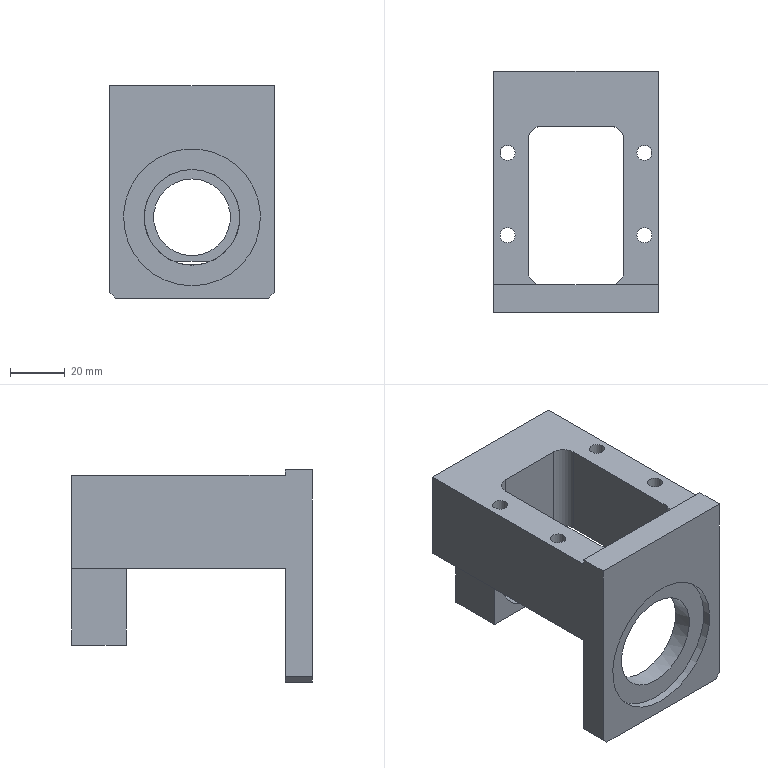Part | NX | 1 solid | 41 faces | box 60 x 88 x 77.5 mm | volume 126887 mm3 | plane 26 | cylinder 15 | commonest cylinder face diameters 5.5 x4 9 x4 10 x4 28 x1 35 x1 50 x1
STEP:
#1=CARTESIAN_POINT('',(-12.738,10.,12.));
#2=VERTEX_POINT('',#1);
#3=CARTESIAN_POINT('',(-12.5,10.,12.));
#4=VERTEX_POINT('',#3);
#5=CARTESIAN_POINT('',(30.,10.,12.));
#6=DIRECTION('',(1.,0.,0.));
#7=VECTOR('',#6,1.);
#8=LINE('',#5,#7);
#9=EDGE_CURVE('',#2,#4,#8,.T.);
#10=ORIENTED_EDGE('',*,*,#9,.T.);
#11=CARTESIAN_POINT('',(-12.5,10.,12.247));
#12=VERTEX_POINT('',#11);
#13=CARTESIAN_POINT('',(-12.5,10.,52.8));
#14=DIRECTION('',(0.,0.,-1.));
#15=VECTOR('',#14,1.);
#16=LINE('',#13,#15);
#17=EDGE_CURVE('',#12,#4,#16,.T.);
#18=ORIENTED_EDGE('',*,*,#17,.F.);
#19=CARTESIAN_POINT('',(0.,10.,0.));
#20=DIRECTION('',(0.,-1.,0.));
#21=DIRECTION('',(0.,0.,-1.));
#22=AXIS2_PLACEMENT_3D('',#19,#20,#21);
#23=CIRCLE('',#22,17.5);
#24=EDGE_CURVE('',#12,#2,#23,.T.);
#25=ORIENTED_EDGE('',*,*,#24,.T.);
#26=EDGE_LOOP('',(#10,#18,#25));
#27=FACE_OUTER_BOUND('',#26,.T.);
#28=CARTESIAN_POINT('',(0.,10.,0.));
#29=DIRECTION('',(0.,1.,0.));
#30=DIRECTION('',(0.,0.,-1.));
#31=AXIS2_PLACEMENT_3D('',#28,#29,#30);
#32=PLANE('',#31);
#33=ADVANCED_FACE('',(#27),#32,.F.);
#34=CARTESIAN_POINT('',(0.,88.,14.));
#35=VERTEX_POINT('',#34);
#36=CARTESIAN_POINT('',(0.,88.,0.));
#37=DIRECTION('',(0.,1.,0.));
#38=DIRECTION('',(0.,0.,1.));
#39=AXIS2_PLACEMENT_3D('',#36,#37,#38);
#40=CIRCLE('',#39,14.);
#41=EDGE_CURVE('',#35,#35,#40,.T.);
#42=ORIENTED_EDGE('',*,*,#41,.T.);
#43=EDGE_LOOP('',(#42));
#44=FACE_BOUND('',#43,.T.);
#45=CARTESIAN_POINT('',(0.,68.,14.));
#46=VERTEX_POINT('',#45);
#47=CARTESIAN_POINT('',(0.,68.,0.));
#48=DIRECTION('',(0.,-1.,0.));
#49=DIRECTION('',(0.,0.,1.));
#50=AXIS2_PLACEMENT_3D('',#47,#48,#49);
#51=CIRCLE('',#50,14.);
#52=EDGE_CURVE('',#46,#46,#51,.T.);
#53=ORIENTED_EDGE('',*,*,#52,.T.);
#54=EDGE_LOOP('',(#53));
#55=FACE_BOUND('',#54,.T.);
#56=CARTESIAN_POINT('',(0.,10.,0.));
#57=DIRECTION('',(0.,1.,0.));
#58=DIRECTION('',(0.,0.,-1.));
#59=AXIS2_PLACEMENT_3D('',#56,#57,#58);
#60=CYLINDRICAL_SURFACE('',#59,14.);
#61=ADVANCED_FACE('',(#44,#55),#60,.F.);
#62=CARTESIAN_POINT('',(12.5,10.,12.));
#63=VERTEX_POINT('',#62);
#64=CARTESIAN_POINT('',(12.738,10.,12.));
#65=VERTEX_POINT('',#64);
#66=CARTESIAN_POINT('',(30.,10.,12.));
#67=DIRECTION('',(1.,0.,0.));
#68=VECTOR('',#67,1.);
#69=LINE('',#66,#68);
#70=EDGE_CURVE('',#63,#65,#69,.T.);
#71=ORIENTED_EDGE('',*,*,#70,.T.);
#72=CARTESIAN_POINT('',(12.5,10.,12.247));
#73=VERTEX_POINT('',#72);
#74=CARTESIAN_POINT('',(0.,10.,0.));
#75=DIRECTION('',(0.,-1.,0.));
#76=DIRECTION('',(0.,0.,-1.));
#77=AXIS2_PLACEMENT_3D('',#74,#75,#76);
#78=CIRCLE('',#77,17.5);
#79=EDGE_CURVE('',#65,#73,#78,.T.);
#80=ORIENTED_EDGE('',*,*,#79,.T.);
#81=CARTESIAN_POINT('',(12.5,10.,52.8));
#82=DIRECTION('',(0.,0.,-1.));
#83=VECTOR('',#82,1.);
#84=LINE('',#81,#83);
#85=EDGE_CURVE('',#73,#63,#84,.T.);
#86=ORIENTED_EDGE('',*,*,#85,.T.);
#87=EDGE_LOOP('',(#71,#80,#86));
#88=FACE_OUTER_BOUND('',#87,.T.);
#89=CARTESIAN_POINT('',(0.,10.,0.));
#90=DIRECTION('',(0.,1.,0.));
#91=DIRECTION('',(0.,0.,-1.));
#92=AXIS2_PLACEMENT_3D('',#89,#90,#91);
#93=PLANE('',#92);
#94=ADVANCED_FACE('',(#88),#93,.F.);
#95=CARTESIAN_POINT('',(-18.,68.,12.));
#96=VERTEX_POINT('',#95);
#97=CARTESIAN_POINT('',(-18.,68.,-16.));
#98=VERTEX_POINT('',#97);
#99=CARTESIAN_POINT('',(-18.,68.,12.));
#100=DIRECTION('',(0.,0.,-1.));
#101=VECTOR('',#100,1.);
#102=LINE('',#99,#101);
#103=EDGE_CURVE('',#96,#98,#102,.T.);
#104=ORIENTED_EDGE('',*,*,#103,.F.);
#105=CARTESIAN_POINT('',(-18.,88.,12.));
#106=VERTEX_POINT('',#105);
#107=CARTESIAN_POINT('',(-18.,10.,12.));
#108=DIRECTION('',(0.,1.,0.));
#109=VECTOR('',#108,1.);
#110=LINE('',#107,#109);
#111=EDGE_CURVE('',#96,#106,#110,.T.);
#112=ORIENTED_EDGE('',*,*,#111,.T.);
#113=CARTESIAN_POINT('',(-18.,88.,-16.));
#114=VERTEX_POINT('',#113);
#115=CARTESIAN_POINT('',(-18.,88.,12.));
#116=DIRECTION('',(0.,0.,-1.));
#117=VECTOR('',#116,1.);
#118=LINE('',#115,#117);
#119=EDGE_CURVE('',#106,#114,#118,.T.);
#120=ORIENTED_EDGE('',*,*,#119,.T.);
#121=CARTESIAN_POINT('',(-18.,10.,-16.));
#122=DIRECTION('',(0.,1.,0.));
#123=VECTOR('',#122,1.);
#124=LINE('',#121,#123);
#125=EDGE_CURVE('',#98,#114,#124,.T.);
#126=ORIENTED_EDGE('',*,*,#125,.F.);
#127=EDGE_LOOP('',(#104,#112,#120,#126));
#128=FACE_OUTER_BOUND('',#127,.T.);
#129=CARTESIAN_POINT('',(-18.,10.,12.));
#130=DIRECTION('',(1.,0.,0.));
#131=DIRECTION('',(0.,0.,1.));
#132=AXIS2_PLACEMENT_3D('',#129,#130,#131);
#133=PLANE('',#132);
#134=ADVANCED_FACE('',(#128),#133,.F.);
#135=CARTESIAN_POINT('',(18.,68.,-16.));
#136=VERTEX_POINT('',#135);
#137=CARTESIAN_POINT('',(18.,68.,12.));
#138=VERTEX_POINT('',#137);
#139=CARTESIAN_POINT('',(18.,68.,-16.));
#140=DIRECTION('',(0.,0.,1.));
#141=VECTOR('',#140,1.);
#142=LINE('',#139,#141);
#143=EDGE_CURVE('',#136,#138,#142,.T.);
#144=ORIENTED_EDGE('',*,*,#143,.F.);
#145=CARTESIAN_POINT('',(18.,88.,-16.));
#146=VERTEX_POINT('',#145);
#147=CARTESIAN_POINT('',(18.,10.,-16.));
#148=DIRECTION('',(0.,1.,0.));
#149=VECTOR('',#148,1.);
#150=LINE('',#147,#149);
#151=EDGE_CURVE('',#136,#146,#150,.T.);
#152=ORIENTED_EDGE('',*,*,#151,.T.);
#153=CARTESIAN_POINT('',(18.,88.,12.));
#154=VERTEX_POINT('',#153);
#155=CARTESIAN_POINT('',(18.,88.,-16.));
#156=DIRECTION('',(0.,0.,1.));
#157=VECTOR('',#156,1.);
#158=LINE('',#155,#157);
#159=EDGE_CURVE('',#146,#154,#158,.T.);
#160=ORIENTED_EDGE('',*,*,#159,.T.);
#161=CARTESIAN_POINT('',(18.,10.,12.));
#162=DIRECTION('',(0.,1.,0.));
#163=VECTOR('',#162,1.);
#164=LINE('',#161,#163);
#165=EDGE_CURVE('',#138,#154,#164,.T.);
#166=ORIENTED_EDGE('',*,*,#165,.F.);
#167=EDGE_LOOP('',(#144,#152,#160,#166));
#168=FACE_OUTER_BOUND('',#167,.T.);
#169=CARTESIAN_POINT('',(18.,10.,-16.));
#170=DIRECTION('',(-1.,0.,0.));
#171=DIRECTION('',(0.,0.,-1.));
#172=AXIS2_PLACEMENT_3D('',#169,#170,#171);
#173=PLANE('',#172);
#174=ADVANCED_FACE('',(#168),#173,.F.);
#175=CARTESIAN_POINT('',(-17.5,63.,12.));
#176=VERTEX_POINT('',#175);
#177=CARTESIAN_POINT('',(-17.5,15.,12.));
#178=VERTEX_POINT('',#177);
#179=CARTESIAN_POINT('',(-17.5,15.,12.));
#180=DIRECTION('',(0.,-1.,0.));
#181=VECTOR('',#180,1.);
#182=LINE('',#179,#181);
#183=EDGE_CURVE('',#176,#178,#182,.T.);
#184=ORIENTED_EDGE('',*,*,#183,.F.);
#185=CARTESIAN_POINT('',(-17.5,63.,46.));
#186=VERTEX_POINT('',#185);
#187=CARTESIAN_POINT('',(-17.5,63.,52.8));
#188=DIRECTION('',(0.,0.,1.));
#189=VECTOR('',#188,1.);
#190=LINE('',#187,#189);
#191=EDGE_CURVE('',#176,#186,#190,.T.);
#192=ORIENTED_EDGE('',*,*,#191,.T.);
#193=CARTESIAN_POINT('',(-17.5,15.,46.));
#194=VERTEX_POINT('',#193);
#195=CARTESIAN_POINT('',(-17.5,10.,46.));
#196=DIRECTION('',(0.,1.,0.));
#197=VECTOR('',#196,1.);
#198=LINE('',#195,#197);
#199=EDGE_CURVE('',#194,#186,#198,.T.);
#200=ORIENTED_EDGE('',*,*,#199,.F.);
#201=CARTESIAN_POINT('',(-17.5,15.,52.8));
#202=DIRECTION('',(0.,0.,1.));
#203=VECTOR('',#202,1.);
#204=LINE('',#201,#203);
#205=EDGE_CURVE('',#178,#194,#204,.T.);
#206=ORIENTED_EDGE('',*,*,#205,.F.);
#207=EDGE_LOOP('',(#184,#192,#200,#206));
#208=FACE_OUTER_BOUND('',#207,.T.);
#209=CARTESIAN_POINT('',(-17.5,15.,52.8));
#210=DIRECTION('',(-1.,0.,0.));
#211=DIRECTION('',(0.,1.,0.));
#212=AXIS2_PLACEMENT_3D('',#209,#210,#211);
#213=PLANE('',#212);
#214=ADVANCED_FACE('',(#208),#213,.F.);
#215=CARTESIAN_POINT('',(17.5,15.,12.));
#216=VERTEX_POINT('',#215);
#217=CARTESIAN_POINT('',(17.5,63.,12.));
#218=VERTEX_POINT('',#217);
#219=CARTESIAN_POINT('',(17.5,63.,12.));
#220=DIRECTION('',(0.,1.,0.));
#221=VECTOR('',#220,1.);
#222=LINE('',#219,#221);
#223=EDGE_CURVE('',#216,#218,#222,.T.);
#224=ORIENTED_EDGE('',*,*,#223,.F.);
#225=CARTESIAN_POINT('',(17.5,15.,46.));
#226=VERTEX_POINT('',#225);
#227=CARTESIAN_POINT('',(17.5,15.,52.8));
#228=DIRECTION('',(0.,0.,1.));
#229=VECTOR('',#228,1.);
#230=LINE('',#227,#229);
#231=EDGE_CURVE('',#216,#226,#230,.T.);
#232=ORIENTED_EDGE('',*,*,#231,.T.);
#233=CARTESIAN_POINT('',(17.5,63.,46.));
#234=VERTEX_POINT('',#233);
#235=CARTESIAN_POINT('',(17.5,10.,46.));
#236=DIRECTION('',(0.,-1.,0.));
#237=VECTOR('',#236,1.);
#238=LINE('',#235,#237);
#239=EDGE_CURVE('',#234,#226,#238,.T.);
#240=ORIENTED_EDGE('',*,*,#239,.F.);
#241=CARTESIAN_POINT('',(17.5,63.,52.8));
#242=DIRECTION('',(0.,0.,1.));
#243=VECTOR('',#242,1.);
#244=LINE('',#241,#243);
#245=EDGE_CURVE('',#218,#234,#244,.T.);
#246=ORIENTED_EDGE('',*,*,#245,.F.);
#247=EDGE_LOOP('',(#224,#232,#240,#246));
#248=FACE_OUTER_BOUND('',#247,.T.);
#249=CARTESIAN_POINT('',(17.5,63.,52.8));
#250=DIRECTION('',(1.,0.,0.));
#251=DIRECTION('',(0.,-1.,0.));
#252=AXIS2_PLACEMENT_3D('',#249,#250,#251);
#253=PLANE('',#252);
#254=ADVANCED_FACE('',(#248),#253,.F.);
#255=CARTESIAN_POINT('',(-12.5,68.,12.));
#256=VERTEX_POINT('',#255);
#257=CARTESIAN_POINT('',(-12.5,63.,12.));
#258=DIRECTION('',(0.,0.,1.));
#259=DIRECTION('',(-1.,0.,0.));
#260=AXIS2_PLACEMENT_3D('',#257,#258,#259);
#261=CIRCLE('',#260,5.);
#262=EDGE_CURVE('',#256,#176,#261,.T.);
#263=ORIENTED_EDGE('',*,*,#262,.F.);
#264=CARTESIAN_POINT('',(-12.5,68.,46.));
#265=VERTEX_POINT('',#264);
#266=CARTESIAN_POINT('',(-12.5,68.,52.8));
#267=DIRECTION('',(0.,0.,1.));
#268=VECTOR('',#267,1.);
#269=LINE('',#266,#268);
#270=EDGE_CURVE('',#256,#265,#269,.T.);
#271=ORIENTED_EDGE('',*,*,#270,.T.);
#272=CARTESIAN_POINT('',(-12.5,63.,46.));
#273=DIRECTION('',(0.,0.,-1.));
#274=DIRECTION('',(-1.,0.,0.));
#275=AXIS2_PLACEMENT_3D('',#272,#273,#274);
#276=CIRCLE('',#275,5.);
#277=EDGE_CURVE('',#186,#265,#276,.T.);
#278=ORIENTED_EDGE('',*,*,#277,.F.);
#279=ORIENTED_EDGE('',*,*,#191,.F.);
#280=EDGE_LOOP('',(#263,#271,#278,#279));
#281=FACE_OUTER_BOUND('',#280,.T.);
#282=CARTESIAN_POINT('',(-12.5,63.,52.8));
#283=DIRECTION('',(0.,0.,-1.));
#284=DIRECTION('',(1.,0.,0.));
#285=AXIS2_PLACEMENT_3D('',#282,#283,#284);
#286=CYLINDRICAL_SURFACE('',#285,5.);
#287=ADVANCED_FACE('',(#281),#286,.F.);
#288=CARTESIAN_POINT('',(12.5,68.,12.));
#289=VERTEX_POINT('',#288);
#290=CARTESIAN_POINT('',(12.5,63.,12.));
#291=DIRECTION('',(0.,0.,1.));
#292=DIRECTION('',(-1.,0.,0.));
#293=AXIS2_PLACEMENT_3D('',#290,#291,#292);
#294=CIRCLE('',#293,5.);
#295=EDGE_CURVE('',#218,#289,#294,.T.);
#296=ORIENTED_EDGE('',*,*,#295,.F.);
#297=ORIENTED_EDGE('',*,*,#245,.T.);
#298=CARTESIAN_POINT('',(12.5,68.,46.));
#299=VERTEX_POINT('',#298);
#300=CARTESIAN_POINT('',(12.5,63.,46.));
#301=DIRECTION('',(0.,0.,-1.));
#302=DIRECTION('',(-1.,0.,0.));
#303=AXIS2_PLACEMENT_3D('',#300,#301,#302);
#304=CIRCLE('',#303,5.);
#305=EDGE_CURVE('',#299,#234,#304,.T.);
#306=ORIENTED_EDGE('',*,*,#305,.F.);
#307=CARTESIAN_POINT('',(12.5,68.,52.8));
#308=DIRECTION('',(0.,0.,1.));
#309=VECTOR('',#308,1.);
#310=LINE('',#307,#309);
#311=EDGE_CURVE('',#289,#299,#310,.T.);
#312=ORIENTED_EDGE('',*,*,#311,.F.);
#313=EDGE_LOOP('',(#296,#297,#306,#312));
#314=FACE_OUTER_BOUND('',#313,.T.);
#315=CARTESIAN_POINT('',(12.5,63.,52.8));
#316=DIRECTION('',(0.,0.,-1.));
#317=DIRECTION('',(1.,0.,0.));
#318=AXIS2_PLACEMENT_3D('',#315,#316,#317);
#319=CYLINDRICAL_SURFACE('',#318,5.);
#320=ADVANCED_FACE('',(#314),#319,.F.);
#321=CARTESIAN_POINT('',(12.5,15.,12.));
#322=DIRECTION('',(0.,0.,1.));
#323=DIRECTION('',(-1.,0.,0.));
#324=AXIS2_PLACEMENT_3D('',#321,#322,#323);
#325=CIRCLE('',#324,5.);
#326=EDGE_CURVE('',#63,#216,#325,.T.);
#327=ORIENTED_EDGE('',*,*,#326,.F.);
#328=ORIENTED_EDGE('',*,*,#85,.F.);
#329=CARTESIAN_POINT('',(12.5,10.,46.));
#330=VERTEX_POINT('',#329);
#331=CARTESIAN_POINT('',(12.5,10.,52.8));
#332=DIRECTION('',(0.,0.,-1.));
#333=VECTOR('',#332,1.);
#334=LINE('',#331,#333);
#335=EDGE_CURVE('',#330,#73,#334,.T.);
#336=ORIENTED_EDGE('',*,*,#335,.F.);
#337=CARTESIAN_POINT('',(12.5,15.,46.));
#338=DIRECTION('',(0.,0.,-1.));
#339=DIRECTION('',(-1.,0.,0.));
#340=AXIS2_PLACEMENT_3D('',#337,#338,#339);
#341=CIRCLE('',#340,5.);
#342=EDGE_CURVE('',#226,#330,#341,.T.);
#343=ORIENTED_EDGE('',*,*,#342,.F.);
#344=ORIENTED_EDGE('',*,*,#231,.F.);
#345=EDGE_LOOP('',(#327,#328,#336,#343,#344));
#346=FACE_OUTER_BOUND('',#345,.T.);
#347=CARTESIAN_POINT('',(12.5,15.,52.8));
#348=DIRECTION('',(0.,0.,-1.));
#349=DIRECTION('',(1.,0.,0.));
#350=AXIS2_PLACEMENT_3D('',#347,#348,#349);
#351=CYLINDRICAL_SURFACE('',#350,5.);
#352=ADVANCED_FACE('',(#346),#351,.F.);
#353=CARTESIAN_POINT('',(-12.5,15.,12.));
#354=DIRECTION('',(0.,0.,1.));
#355=DIRECTION('',(-1.,0.,0.));
#356=AXIS2_PLACEMENT_3D('',#353,#354,#355);
#357=CIRCLE('',#356,5.);
#358=EDGE_CURVE('',#178,#4,#357,.T.);
#359=ORIENTED_EDGE('',*,*,#358,.F.);
#360=ORIENTED_EDGE('',*,*,#205,.T.);
#361=CARTESIAN_POINT('',(-12.5,10.,46.));
#362=VERTEX_POINT('',#361);
#363=CARTESIAN_POINT('',(-12.5,15.,46.));
#364=DIRECTION('',(0.,0.,-1.));
#365=DIRECTION('',(-1.,0.,0.));
#366=AXIS2_PLACEMENT_3D('',#363,#364,#365);
#367=CIRCLE('',#366,5.);
#368=EDGE_CURVE('',#362,#194,#367,.T.);
#369=ORIENTED_EDGE('',*,*,#368,.F.);
#370=CARTESIAN_POINT('',(-12.5,10.,52.8));
#371=DIRECTION('',(0.,0.,-1.));
#372=VECTOR('',#371,1.);
#373=LINE('',#370,#372);
#374=EDGE_CURVE('',#362,#12,#373,.T.);
#375=ORIENTED_EDGE('',*,*,#374,.T.);
#376=ORIENTED_EDGE('',*,*,#17,.T.);
#377=EDGE_LOOP('',(#359,#360,#369,#375,#376));
#378=FACE_OUTER_BOUND('',#377,.T.);
#379=CARTESIAN_POINT('',(-12.5,15.,52.8));
#380=DIRECTION('',(0.,0.,-1.));
#381=DIRECTION('',(1.,0.,0.));
#382=AXIS2_PLACEMENT_3D('',#379,#380,#381);
#383=CYLINDRICAL_SURFACE('',#382,5.);
#384=ADVANCED_FACE('',(#378),#383,.F.);
#385=CARTESIAN_POINT('',(22.25,28.2,46.));
#386=VERTEX_POINT('',#385);
#387=CARTESIAN_POINT('',(25.,28.2,46.));
#388=DIRECTION('',(0.,0.,1.));
#389=DIRECTION('',(-1.,0.,0.));
#390=AXIS2_PLACEMENT_3D('',#387,#388,#389);
#391=CIRCLE('',#390,2.75);
#392=EDGE_CURVE('',#386,#386,#391,.T.);
#393=ORIENTED_EDGE('',*,*,#392,.F.);
#394=EDGE_LOOP('',(#393));
#395=FACE_BOUND('',#394,.T.);
#396=CARTESIAN_POINT('',(-27.75,58.2,46.));
#397=VERTEX_POINT('',#396);
#398=CARTESIAN_POINT('',(-25.,58.2,46.));
#399=DIRECTION('',(0.,0.,1.));
#400=DIRECTION('',(-1.,0.,0.));
#401=AXIS2_PLACEMENT_3D('',#398,#399,#400);
#402=CIRCLE('',#401,2.75);
#403=EDGE_CURVE('',#397,#397,#402,.T.);
#404=ORIENTED_EDGE('',*,*,#403,.F.);
#405=EDGE_LOOP('',(#404));
#406=FACE_BOUND('',#405,.T.);
#407=ORIENTED_EDGE('',*,*,#239,.T.);
#408=ORIENTED_EDGE('',*,*,#342,.T.);
#409=CARTESIAN_POINT('',(30.,10.,46.));
#410=VERTEX_POINT('',#409);
#411=CARTESIAN_POINT('',(30.,10.,46.));
#412=DIRECTION('',(-1.,0.,0.));
#413=VECTOR('',#412,1.);
#414=LINE('',#411,#413);
#415=EDGE_CURVE('',#410,#330,#414,.T.);
#416=ORIENTED_EDGE('',*,*,#415,.F.);
#417=CARTESIAN_POINT('',(30.,88.,46.));
#418=VERTEX_POINT('',#417);
#419=CARTESIAN_POINT('',(30.,10.,46.));
#420=DIRECTION('',(0.,1.,0.));
#421=VECTOR('',#420,1.);
#422=LINE('',#419,#421);
#423=EDGE_CURVE('',#410,#418,#422,.T.);
#424=ORIENTED_EDGE('',*,*,#423,.T.);
#425=CARTESIAN_POINT('',(-30.,88.,46.));
#426=VERTEX_POINT('',#425);
#427=CARTESIAN_POINT('',(30.,88.,46.));
#428=DIRECTION('',(-1.,0.,0.));
#429=VECTOR('',#428,1.);
#430=LINE('',#427,#429);
#431=EDGE_CURVE('',#418,#426,#430,.T.);
#432=ORIENTED_EDGE('',*,*,#431,.T.);
#433=CARTESIAN_POINT('',(-30.,10.,46.));
#434=VERTEX_POINT('',#433);
#435=CARTESIAN_POINT('',(-30.,10.,46.));
#436=DIRECTION('',(0.,1.,0.));
#437=VECTOR('',#436,1.);
#438=LINE('',#435,#437);
#439=EDGE_CURVE('',#434,#426,#438,.T.);
#440=ORIENTED_EDGE('',*,*,#439,.F.);
#441=CARTESIAN_POINT('',(30.,10.,46.));
#442=DIRECTION('',(-1.,0.,0.));
#443=VECTOR('',#442,1.);
#444=LINE('',#441,#443);
#445=EDGE_CURVE('',#362,#434,#444,.T.);
#446=ORIENTED_EDGE('',*,*,#445,.F.);
#447=ORIENTED_EDGE('',*,*,#368,.T.);
#448=ORIENTED_EDGE('',*,*,#199,.T.);
#449=ORIENTED_EDGE('',*,*,#277,.T.);
#450=CARTESIAN_POINT('',(30.,68.,46.));
#451=DIRECTION('',(1.,0.,0.));
#452=VECTOR('',#451,1.);
#453=LINE('',#450,#452);
#454=EDGE_CURVE('',#265,#299,#453,.T.);
#455=ORIENTED_EDGE('',*,*,#454,.T.);
#456=ORIENTED_EDGE('',*,*,#305,.T.);
#457=EDGE_LOOP('',(#407,#408,#416,#424,#432,#440,#446,#447,#448,#449,#455,#456));
#458=FACE_BOUND('',#457,.T.);
#459=CARTESIAN_POINT('',(22.25,58.2,46.));
#460=VERTEX_POINT('',#459);
#461=CARTESIAN_POINT('',(25.,58.2,46.));
#462=DIRECTION('',(0.,0.,1.));
#463=DIRECTION('',(-1.,0.,0.));
#464=AXIS2_PLACEMENT_3D('',#461,#462,#463);
#465=CIRCLE('',#464,2.75);
#466=EDGE_CURVE('',#460,#460,#465,.T.);
#467=ORIENTED_EDGE('',*,*,#466,.F.);
#468=EDGE_LOOP('',(#467));
#469=FACE_BOUND('',#468,.T.);
#470=CARTESIAN_POINT('',(-27.75,28.2,46.));
#471=VERTEX_POINT('',#470);
#472=CARTESIAN_POINT('',(-25.,28.2,46.));
#473=DIRECTION('',(0.,0.,-1.));
#474=DIRECTION('',(-1.,0.,0.));
#475=AXIS2_PLACEMENT_3D('',#472,#473,#474);
#476=CIRCLE('',#475,2.75);
#477=EDGE_CURVE('',#471,#471,#476,.T.);
#478=ORIENTED_EDGE('',*,*,#477,.T.);
#479=EDGE_LOOP('',(#478));
#480=FACE_BOUND('',#479,.T.);
#481=CARTESIAN_POINT('',(30.,10.,46.));
#482=DIRECTION('',(0.,0.,-1.));
#483=DIRECTION('',(1.,0.,0.));
#484=AXIS2_PLACEMENT_3D('',#481,#482,#483);
#485=PLANE('',#484);
#486=ADVANCED_FACE('',(#395,#406,#458,#469,#480),#485,.F.);
#487=CARTESIAN_POINT('',(30.,88.,12.));
#488=VERTEX_POINT('',#487);
#489=CARTESIAN_POINT('',(30.,88.,12.));
#490=DIRECTION('',(0.,0.,1.));
#491=VECTOR('',#490,1.);
#492=LINE('',#489,#491);
#493=EDGE_CURVE('',#488,#418,#492,.T.);
#494=ORIENTED_EDGE('',*,*,#493,.T.);
#495=ORIENTED_EDGE('',*,*,#423,.F.);
#496=CARTESIAN_POINT('',(30.,10.,48.));
#497=VERTEX_POINT('',#496);
#498=CARTESIAN_POINT('',(30.,10.,48.));
#499=DIRECTION('',(0.,0.,-1.));
#500=VECTOR('',#499,1.);
#501=LINE('',#498,#500);
#502=EDGE_CURVE('',#497,#410,#501,.T.);
#503=ORIENTED_EDGE('',*,*,#502,.F.);
#504=CARTESIAN_POINT('',(30.,0.,48.));
#505=VERTEX_POINT('',#504);
#506=CARTESIAN_POINT('',(30.,10.,48.));
#507=DIRECTION('',(0.,-1.,0.));
#508=VECTOR('',#507,1.);
#509=LINE('',#506,#508);
#510=EDGE_CURVE('',#497,#505,#509,.T.);
#511=ORIENTED_EDGE('',*,*,#510,.T.);
#512=CARTESIAN_POINT('',(30.,0.,-27.5));
#513=VERTEX_POINT('',#512);
#514=CARTESIAN_POINT('',(30.,0.,48.));
#515=DIRECTION('',(0.,0.,-1.));
#516=VECTOR('',#515,1.);
#517=LINE('',#514,#516);
#518=EDGE_CURVE('',#505,#513,#517,.T.);
#519=ORIENTED_EDGE('',*,*,#518,.T.);
#520=CARTESIAN_POINT('',(30.,10.,-27.5));
#521=VERTEX_POINT('',#520);
#522=CARTESIAN_POINT('',(30.,10.,-27.5));
#523=DIRECTION('',(0.,-1.,0.));
#524=VECTOR('',#523,1.);
#525=LINE('',#522,#524);
#526=EDGE_CURVE('',#521,#513,#525,.T.);
#527=ORIENTED_EDGE('',*,*,#526,.F.);
#528=CARTESIAN_POINT('',(30.,10.,12.));
#529=VERTEX_POINT('',#528);
#530=CARTESIAN_POINT('',(30.,10.,48.));
#531=DIRECTION('',(0.,0.,-1.));
#532=VECTOR('',#531,1.);
#533=LINE('',#530,#532);
#534=EDGE_CURVE('',#529,#521,#533,.T.);
#535=ORIENTED_EDGE('',*,*,#534,.F.);
#536=CARTESIAN_POINT('',(30.,10.,12.));
#537=DIRECTION('',(0.,1.,0.));
#538=VECTOR('',#537,1.);
#539=LINE('',#536,#538);
#540=EDGE_CURVE('',#529,#488,#539,.T.);
#541=ORIENTED_EDGE('',*,*,#540,.T.);
#542=EDGE_LOOP('',(#494,#495,#503,#511,#519,#527,#535,#541));
#543=FACE_OUTER_BOUND('',#542,.T.);
#544=CARTESIAN_POINT('',(30.,10.,12.));
#545=DIRECTION('',(-1.,0.,0.));
#546=DIRECTION('',(0.,0.,-1.));
#547=AXIS2_PLACEMENT_3D('',#544,#545,#546);
#548=PLANE('',#547);
#549=ADVANCED_FACE('',(#543),#548,.F.);
#550=CARTESIAN_POINT('',(-30.,88.,12.));
#551=VERTEX_POINT('',#550);
#552=CARTESIAN_POINT('',(-30.,88.,46.));
#553=DIRECTION('',(0.,0.,-1.));
#554=VECTOR('',#553,1.);
#555=LINE('',#552,#554);
#556=EDGE_CURVE('',#426,#551,#555,.T.);
#557=ORIENTED_EDGE('',*,*,#556,.T.);
#558=CARTESIAN_POINT('',(-30.,10.,12.));
#559=VERTEX_POINT('',#558);
#560=CARTESIAN_POINT('',(-30.,10.,12.));
#561=DIRECTION('',(0.,1.,0.));
#562=VECTOR('',#561,1.);
#563=LINE('',#560,#562);
#564=EDGE_CURVE('',#559,#551,#563,.T.);
#565=ORIENTED_EDGE('',*,*,#564,.F.);
#566=CARTESIAN_POINT('',(-30.,10.,-27.5));
#567=VERTEX_POINT('',#566);
#568=CARTESIAN_POINT('',(-30.,10.,-27.5));
#569=DIRECTION('',(0.,0.,1.));
#570=VECTOR('',#569,1.);
#571=LINE('',#568,#570);
#572=EDGE_CURVE('',#567,#559,#571,.T.);
#573=ORIENTED_EDGE('',*,*,#572,.F.);
#574=CARTESIAN_POINT('',(-30.,0.,-27.5));
#575=VERTEX_POINT('',#574);
#576=CARTESIAN_POINT('',(-30.,10.,-27.5));
#577=DIRECTION('',(0.,-1.,0.));
#578=VECTOR('',#577,1.);
#579=LINE('',#576,#578);
#580=EDGE_CURVE('',#567,#575,#579,.T.);
#581=ORIENTED_EDGE('',*,*,#580,.T.);
#582=CARTESIAN_POINT('',(-30.,0.,48.));
#583=VERTEX_POINT('',#582);
#584=CARTESIAN_POINT('',(-30.,0.,-27.5));
#585=DIRECTION('',(0.,0.,1.));
#586=VECTOR('',#585,1.);
#587=LINE('',#584,#586);
#588=EDGE_CURVE('',#575,#583,#587,.T.);
#589=ORIENTED_EDGE('',*,*,#588,.T.);
#590=CARTESIAN_POINT('',(-30.,10.,48.));
#591=VERTEX_POINT('',#590);
#592=CARTESIAN_POINT('',(-30.,10.,48.));
#593=DIRECTION('',(0.,-1.,0.));
#594=VECTOR('',#593,1.);
#595=LINE('',#592,#594);
#596=EDGE_CURVE('',#591,#583,#595,.T.);
#597=ORIENTED_EDGE('',*,*,#596,.F.);
#598=CARTESIAN_POINT('',(-30.,10.,-27.5));
#599=DIRECTION('',(0.,0.,1.));
#600=VECTOR('',#599,1.);
#601=LINE('',#598,#600);
#602=EDGE_CURVE('',#434,#591,#601,.T.);
#603=ORIENTED_EDGE('',*,*,#602,.F.);
#604=ORIENTED_EDGE('',*,*,#439,.T.);
#605=EDGE_LOOP('',(#557,#565,#573,#581,#589,#597,#603,#604));
#606=FACE_OUTER_BOUND('',#605,.T.);
#607=CARTESIAN_POINT('',(-30.,10.,46.));
#608=DIRECTION('',(1.,0.,0.));
#609=DIRECTION('',(0.,0.,1.));
#610=AXIS2_PLACEMENT_3D('',#607,#608,#609);
#611=PLANE('',#610);
#612=ADVANCED_FACE('',(#606),#611,.F.);
#613=CARTESIAN_POINT('',(-20.5,58.2,12.));
#614=VERTEX_POINT('',#613);
#615=CARTESIAN_POINT('',(-25.,58.2,12.));
#616=DIRECTION('',(0.,0.,1.));
#617=DIRECTION('',(1.,0.,0.));
#618=AXIS2_PLACEMENT_3D('',#615,#616,#617);
#619=CIRCLE('',#618,4.5);
#620=EDGE_CURVE('',#614,#614,#619,.T.);
#621=ORIENTED_EDGE('',*,*,#620,.T.);
#622=EDGE_LOOP('',(#621));
#623=FACE_BOUND('',#622,.T.);
#624=CARTESIAN_POINT('',(-20.5,28.2,12.));
#625=VERTEX_POINT('',#624);
#626=CARTESIAN_POINT('',(-25.,28.2,12.));
#627=DIRECTION('',(0.,0.,1.));
#628=DIRECTION('',(1.,0.,0.));
#629=AXIS2_PLACEMENT_3D('',#626,#627,#628);
#630=CIRCLE('',#629,4.5);
#631=EDGE_CURVE('',#625,#625,#630,.T.);
#632=ORIENTED_EDGE('',*,*,#631,.T.);
#633=EDGE_LOOP('',(#632));
#634=FACE_BOUND('',#633,.T.);
#635=ORIENTED_EDGE('',*,*,#564,.T.);
#636=CARTESIAN_POINT('',(-30.,88.,12.));
#637=DIRECTION('',(1.,0.,0.));
#638=VECTOR('',#637,1.);
#639=LINE('',#636,#638);
#640=EDGE_CURVE('',#551,#106,#639,.T.);
#641=ORIENTED_EDGE('',*,*,#640,.T.);
#642=ORIENTED_EDGE('',*,*,#111,.F.);
#643=CARTESIAN_POINT('',(-50.,68.,12.));
#644=DIRECTION('',(1.,0.,0.));
#645=VECTOR('',#644,1.);
#646=LINE('',#643,#645);
#647=EDGE_CURVE('',#96,#256,#646,.T.);
#648=ORIENTED_EDGE('',*,*,#647,.T.);
#649=ORIENTED_EDGE('',*,*,#262,.T.);
#650=ORIENTED_EDGE('',*,*,#183,.T.);
#651=ORIENTED_EDGE('',*,*,#358,.T.);
#652=ORIENTED_EDGE('',*,*,#9,.F.);
#653=CARTESIAN_POINT('',(-30.,10.,12.));
#654=DIRECTION('',(1.,0.,0.));
#655=VECTOR('',#654,1.);
#656=LINE('',#653,#655);
#657=EDGE_CURVE('',#559,#2,#656,.T.);
#658=ORIENTED_EDGE('',*,*,#657,.F.);
#659=EDGE_LOOP('',(#635,#641,#642,#648,#649,#650,#651,#652,#658));
#660=FACE_BOUND('',#659,.T.);
#661=CARTESIAN_POINT('',(-30.,10.,12.));
#662=DIRECTION('',(0.,0.,1.));
#663=DIRECTION('',(-1.,0.,0.));
#664=AXIS2_PLACEMENT_3D('',#661,#662,#663);
#665=PLANE('',#664);
#666=ADVANCED_FACE('',(#623,#634,#660),#665,.F.);
#667=ORIENTED_EDGE('',*,*,#151,.F.);
#668=CARTESIAN_POINT('',(-18.,68.,-16.));
#669=DIRECTION('',(-1.,0.,0.));
#670=VECTOR('',#669,1.);
#671=LINE('',#668,#670);
#672=EDGE_CURVE('',#136,#98,#671,.T.);
#673=ORIENTED_EDGE('',*,*,#672,.T.);
#674=ORIENTED_EDGE('',*,*,#125,.T.);
#675=CARTESIAN_POINT('',(-18.,88.,-16.));
#676=DIRECTION('',(1.,0.,0.));
#677=VECTOR('',#676,1.);
#678=LINE('',#675,#677);
#679=EDGE_CURVE('',#114,#146,#678,.T.);
#680=ORIENTED_EDGE('',*,*,#679,.T.);
#681=EDGE_LOOP('',(#667,#673,#674,#680));
#682=FACE_OUTER_BOUND('',#681,.T.);
#683=CARTESIAN_POINT('',(-18.,10.,-16.));
#684=DIRECTION('',(0.,0.,1.));
#685=DIRECTION('',(-1.,0.,0.));
#686=AXIS2_PLACEMENT_3D('',#683,#684,#685);
#687=PLANE('',#686);
#688=ADVANCED_FACE('',(#682),#687,.F.);
#689=CARTESIAN_POINT('',(29.5,58.2,12.));
#690=VERTEX_POINT('',#689);
#691=CARTESIAN_POINT('',(25.,58.2,12.));
#692=DIRECTION('',(0.,0.,1.));
#693=DIRECTION('',(1.,0.,0.));
#694=AXIS2_PLACEMENT_3D('',#691,#692,#693);
#695=CIRCLE('',#694,4.5);
#696=EDGE_CURVE('',#690,#690,#695,.T.);
#697=ORIENTED_EDGE('',*,*,#696,.T.);
#698=EDGE_LOOP('',(#697));
#699=FACE_BOUND('',#698,.T.);
#700=CARTESIAN_POINT('',(29.5,28.2,12.));
#701=VERTEX_POINT('',#700);
#702=CARTESIAN_POINT('',(25.,28.2,12.));
#703=DIRECTION('',(0.,0.,1.));
#704=DIRECTION('',(1.,0.,0.));
#705=AXIS2_PLACEMENT_3D('',#702,#703,#704);
#706=CIRCLE('',#705,4.5);
#707=EDGE_CURVE('',#701,#701,#706,.T.);
#708=ORIENTED_EDGE('',*,*,#707,.T.);
#709=EDGE_LOOP('',(#708));
#710=FACE_BOUND('',#709,.T.);
#711=CARTESIAN_POINT('',(18.,10.,12.));
#712=DIRECTION('',(1.,0.,0.));
#713=VECTOR('',#712,1.);
#714=LINE('',#711,#713);
#715=EDGE_CURVE('',#65,#529,#714,.T.);
#716=ORIENTED_EDGE('',*,*,#715,.F.);
#717=ORIENTED_EDGE('',*,*,#70,.F.);
#718=ORIENTED_EDGE('',*,*,#326,.T.);
#719=ORIENTED_EDGE('',*,*,#223,.T.);
#720=ORIENTED_EDGE('',*,*,#295,.T.);
#721=CARTESIAN_POINT('',(-50.,68.,12.));
#722=DIRECTION('',(1.,0.,0.));
#723=VECTOR('',#722,1.);
#724=LINE('',#721,#723);
#725=EDGE_CURVE('',#289,#138,#724,.T.);
#726=ORIENTED_EDGE('',*,*,#725,.T.);
#727=ORIENTED_EDGE('',*,*,#165,.T.);
#728=CARTESIAN_POINT('',(18.,88.,12.));
#729=DIRECTION('',(1.,0.,0.));
#730=VECTOR('',#729,1.);
#731=LINE('',#728,#730);
#732=EDGE_CURVE('',#154,#488,#731,.T.);
#733=ORIENTED_EDGE('',*,*,#732,.T.);
#734=ORIENTED_EDGE('',*,*,#540,.F.);
#735=EDGE_LOOP('',(#716,#717,#718,#719,#720,#726,#727,#733,#734));
#736=FACE_BOUND('',#735,.T.);
#737=CARTESIAN_POINT('',(18.,10.,12.));
#738=DIRECTION('',(0.,0.,1.));
#739=DIRECTION('',(-1.,0.,0.));
#740=AXIS2_PLACEMENT_3D('',#737,#738,#739);
#741=PLANE('',#740);
#742=ADVANCED_FACE('',(#699,#710,#736),#741,.F.);
#743=ORIENTED_EDGE('',*,*,#493,.F.);
#744=ORIENTED_EDGE('',*,*,#732,.F.);
#745=ORIENTED_EDGE('',*,*,#159,.F.);
#746=ORIENTED_EDGE('',*,*,#679,.F.);
#747=ORIENTED_EDGE('',*,*,#119,.F.);
#748=ORIENTED_EDGE('',*,*,#640,.F.);
#749=ORIENTED_EDGE('',*,*,#556,.F.);
#750=ORIENTED_EDGE('',*,*,#431,.F.);
#751=EDGE_LOOP('',(#743,#744,#745,#746,#747,#748,#749,#750));
#752=FACE_BOUND('',#751,.T.);
#753=ORIENTED_EDGE('',*,*,#41,.F.);
#754=EDGE_LOOP('',(#753));
#755=FACE_BOUND('',#754,.T.);
#756=CARTESIAN_POINT('',(0.,88.,0.));
#757=DIRECTION('',(0.,1.,0.));
#758=DIRECTION('',(0.,0.,-1.));
#759=AXIS2_PLACEMENT_3D('',#756,#757,#758);
#760=PLANE('',#759);
#761=ADVANCED_FACE('',(#752,#755),#760,.T.);
#762=CARTESIAN_POINT('',(-30.,10.,48.));
#763=DIRECTION('',(1.,0.,0.));
#764=VECTOR('',#763,1.);
#765=LINE('',#762,#764);
#766=EDGE_CURVE('',#591,#497,#765,.T.);
#767=ORIENTED_EDGE('',*,*,#766,.T.);
#768=ORIENTED_EDGE('',*,*,#502,.T.);
#769=ORIENTED_EDGE('',*,*,#415,.T.);
#770=ORIENTED_EDGE('',*,*,#335,.T.);
#771=CARTESIAN_POINT('',(0.,10.,0.));
#772=DIRECTION('',(0.,-1.,0.));
#773=DIRECTION('',(0.,0.,-1.));
#774=AXIS2_PLACEMENT_3D('',#771,#772,#773);
#775=CIRCLE('',#774,17.5);
#776=EDGE_CURVE('',#73,#12,#775,.T.);
#777=ORIENTED_EDGE('',*,*,#776,.T.);
#778=ORIENTED_EDGE('',*,*,#374,.F.);
#779=ORIENTED_EDGE('',*,*,#445,.T.);
#780=ORIENTED_EDGE('',*,*,#602,.T.);
#781=EDGE_LOOP('',(#767,#768,#769,#770,#777,#778,#779,#780));
#782=FACE_OUTER_BOUND('',#781,.T.);
#783=CARTESIAN_POINT('',(0.,10.,0.));
#784=DIRECTION('',(0.,-1.,0.));
#785=DIRECTION('',(0.,0.,1.));
#786=AXIS2_PLACEMENT_3D('',#783,#784,#785);
#787=PLANE('',#786);
#788=ADVANCED_FACE('',(#782),#787,.F.);
#789=CARTESIAN_POINT('',(0.,10.,0.));
#790=DIRECTION('',(0.,-1.,0.));
#791=DIRECTION('',(0.,0.,-1.));
#792=AXIS2_PLACEMENT_3D('',#789,#790,#791);
#793=CIRCLE('',#792,17.5);
#794=EDGE_CURVE('',#2,#65,#793,.T.);
#795=ORIENTED_EDGE('',*,*,#794,.T.);
#796=ORIENTED_EDGE('',*,*,#715,.T.);
#797=ORIENTED_EDGE('',*,*,#534,.T.);
#798=CARTESIAN_POINT('',(28.,10.,-29.5));
#799=VERTEX_POINT('',#798);
#800=CARTESIAN_POINT('',(30.,10.,-27.5));
#801=DIRECTION('',(-0.7071,0.,-0.7071));
#802=VECTOR('',#801,1.);
#803=LINE('',#800,#802);
#804=EDGE_CURVE('',#521,#799,#803,.T.);
#805=ORIENTED_EDGE('',*,*,#804,.T.);
#806=CARTESIAN_POINT('',(-28.,10.,-29.5));
#807=VERTEX_POINT('',#806);
#808=CARTESIAN_POINT('',(28.,10.,-29.5));
#809=DIRECTION('',(-1.,0.,0.));
#810=VECTOR('',#809,1.);
#811=LINE('',#808,#810);
#812=EDGE_CURVE('',#799,#807,#811,.T.);
#813=ORIENTED_EDGE('',*,*,#812,.T.);
#814=CARTESIAN_POINT('',(-28.,10.,-29.5));
#815=DIRECTION('',(-0.7071,0.,0.7071));
#816=VECTOR('',#815,1.);
#817=LINE('',#814,#816);
#818=EDGE_CURVE('',#807,#567,#817,.T.);
#819=ORIENTED_EDGE('',*,*,#818,.T.);
#820=ORIENTED_EDGE('',*,*,#572,.T.);
#821=ORIENTED_EDGE('',*,*,#657,.T.);
#822=EDGE_LOOP('',(#795,#796,#797,#805,#813,#819,#820,#821));
#823=FACE_OUTER_BOUND('',#822,.T.);
#824=CARTESIAN_POINT('',(0.,10.,0.));
#825=DIRECTION('',(0.,-1.,0.));
#826=DIRECTION('',(0.,0.,1.));
#827=AXIS2_PLACEMENT_3D('',#824,#825,#826);
#828=PLANE('',#827);
#829=ADVANCED_FACE('',(#823),#828,.F.);
#830=CARTESIAN_POINT('',(28.,0.,-29.5));
#831=VERTEX_POINT('',#830);
#832=CARTESIAN_POINT('',(30.,0.,-27.5));
#833=DIRECTION('',(-0.7071,0.,-0.7071));
#834=VECTOR('',#833,1.);
#835=LINE('',#832,#834);
#836=EDGE_CURVE('',#513,#831,#835,.T.);
#837=ORIENTED_EDGE('',*,*,#836,.T.);
#838=CARTESIAN_POINT('',(28.,10.,-29.5));
#839=DIRECTION('',(0.,-1.,0.));
#840=VECTOR('',#839,1.);
#841=LINE('',#838,#840);
#842=EDGE_CURVE('',#799,#831,#841,.T.);
#843=ORIENTED_EDGE('',*,*,#842,.F.);
#844=ORIENTED_EDGE('',*,*,#804,.F.);
#845=ORIENTED_EDGE('',*,*,#526,.T.);
#846=EDGE_LOOP('',(#837,#843,#844,#845));
#847=FACE_OUTER_BOUND('',#846,.T.);
#848=CARTESIAN_POINT('',(30.,10.,-27.5));
#849=DIRECTION('',(-0.7071,0.,0.7071));
#850=DIRECTION('',(-0.7071,0.,-0.7071));
#851=AXIS2_PLACEMENT_3D('',#848,#849,#850);
#852=PLANE('',#851);
#853=ADVANCED_FACE('',(#847),#852,.F.);
#854=CARTESIAN_POINT('',(-28.,0.,-29.5));
#855=VERTEX_POINT('',#854);
#856=CARTESIAN_POINT('',(28.,0.,-29.5));
#857=DIRECTION('',(-1.,0.,0.));
#858=VECTOR('',#857,1.);
#859=LINE('',#856,#858);
#860=EDGE_CURVE('',#831,#855,#859,.T.);
#861=ORIENTED_EDGE('',*,*,#860,.T.);
#862=CARTESIAN_POINT('',(-28.,10.,-29.5));
#863=DIRECTION('',(0.,-1.,0.));
#864=VECTOR('',#863,1.);
#865=LINE('',#862,#864);
#866=EDGE_CURVE('',#807,#855,#865,.T.);
#867=ORIENTED_EDGE('',*,*,#866,.F.);
#868=ORIENTED_EDGE('',*,*,#812,.F.);
#869=ORIENTED_EDGE('',*,*,#842,.T.);
#870=EDGE_LOOP('',(#861,#867,#868,#869));
#871=FACE_OUTER_BOUND('',#870,.T.);
#872=CARTESIAN_POINT('',(28.,10.,-29.5));
#873=DIRECTION('',(0.,0.,1.));
#874=DIRECTION('',(-1.,0.,0.));
#875=AXIS2_PLACEMENT_3D('',#872,#873,#874);
#876=PLANE('',#875);
#877=ADVANCED_FACE('',(#871),#876,.F.);
#878=CARTESIAN_POINT('',(-28.,0.,-29.5));
#879=DIRECTION('',(-0.7071,0.,0.7071));
#880=VECTOR('',#879,1.);
#881=LINE('',#878,#880);
#882=EDGE_CURVE('',#855,#575,#881,.T.);
#883=ORIENTED_EDGE('',*,*,#882,.T.);
#884=ORIENTED_EDGE('',*,*,#580,.F.);
#885=ORIENTED_EDGE('',*,*,#818,.F.);
#886=ORIENTED_EDGE('',*,*,#866,.T.);
#887=EDGE_LOOP('',(#883,#884,#885,#886));
#888=FACE_OUTER_BOUND('',#887,.T.);
#889=CARTESIAN_POINT('',(-28.,10.,-29.5));
#890=DIRECTION('',(0.7071,0.,0.7071));
#891=DIRECTION('',(-0.7071,0.,0.7071));
#892=AXIS2_PLACEMENT_3D('',#889,#890,#891);
#893=PLANE('',#892);
#894=ADVANCED_FACE('',(#888),#893,.F.);
#895=CARTESIAN_POINT('',(-30.,0.,48.));
#896=DIRECTION('',(1.,0.,0.));
#897=VECTOR('',#896,1.);
#898=LINE('',#895,#897);
#899=EDGE_CURVE('',#583,#505,#898,.T.);
#900=ORIENTED_EDGE('',*,*,#899,.T.);
#901=ORIENTED_EDGE('',*,*,#510,.F.);
#902=ORIENTED_EDGE('',*,*,#766,.F.);
#903=ORIENTED_EDGE('',*,*,#596,.T.);
#904=EDGE_LOOP('',(#900,#901,#902,#903));
#905=FACE_OUTER_BOUND('',#904,.T.);
#906=CARTESIAN_POINT('',(-30.,10.,48.));
#907=DIRECTION('',(0.,0.,-1.));
#908=DIRECTION('',(1.,0.,0.));
#909=AXIS2_PLACEMENT_3D('',#906,#907,#908);
#910=PLANE('',#909);
#911=ADVANCED_FACE('',(#905),#910,.F.);
#912=CARTESIAN_POINT('',(0.,3.,17.5));
#913=VERTEX_POINT('',#912);
#914=CARTESIAN_POINT('',(0.,3.,0.));
#915=DIRECTION('',(0.,-1.,0.));
#916=DIRECTION('',(0.,0.,1.));
#917=AXIS2_PLACEMENT_3D('',#914,#915,#916);
#918=CIRCLE('',#917,17.5);
#919=EDGE_CURVE('',#913,#913,#918,.T.);
#920=ORIENTED_EDGE('',*,*,#919,.T.);
#921=EDGE_LOOP('',(#920));
#922=FACE_BOUND('',#921,.T.);
#923=ORIENTED_EDGE('',*,*,#79,.F.);
#924=ORIENTED_EDGE('',*,*,#794,.F.);
#925=ORIENTED_EDGE('',*,*,#24,.F.);
#926=ORIENTED_EDGE('',*,*,#776,.F.);
#927=EDGE_LOOP('',(#923,#924,#925,#926));
#928=FACE_BOUND('',#927,.T.);
#929=CARTESIAN_POINT('',(0.,10.,0.));
#930=DIRECTION('',(0.,-1.,0.));
#931=DIRECTION('',(0.,0.,1.));
#932=AXIS2_PLACEMENT_3D('',#929,#930,#931);
#933=CYLINDRICAL_SURFACE('',#932,17.5);
#934=ADVANCED_FACE('',(#922,#928),#933,.F.);
#935=CARTESIAN_POINT('',(0.,0.,-25.));
#936=VERTEX_POINT('',#935);
#937=CARTESIAN_POINT('',(0.,0.,0.));
#938=DIRECTION('',(0.,1.,0.));
#939=DIRECTION('',(0.,0.,-1.));
#940=AXIS2_PLACEMENT_3D('',#937,#938,#939);
#941=CIRCLE('',#940,25.);
#942=EDGE_CURVE('',#936,#936,#941,.T.);
#943=ORIENTED_EDGE('',*,*,#942,.T.);
#944=EDGE_LOOP('',(#943));
#945=FACE_BOUND('',#944,.T.);
#946=ORIENTED_EDGE('',*,*,#518,.F.);
#947=ORIENTED_EDGE('',*,*,#899,.F.);
#948=ORIENTED_EDGE('',*,*,#588,.F.);
#949=ORIENTED_EDGE('',*,*,#882,.F.);
#950=ORIENTED_EDGE('',*,*,#860,.F.);
#951=ORIENTED_EDGE('',*,*,#836,.F.);
#952=EDGE_LOOP('',(#946,#947,#948,#949,#950,#951));
#953=FACE_BOUND('',#952,.T.);
#954=CARTESIAN_POINT('',(0.,0.,0.));
#955=DIRECTION('',(0.,-1.,0.));
#956=DIRECTION('',(0.,0.,1.));
#957=AXIS2_PLACEMENT_3D('',#954,#955,#956);
#958=PLANE('',#957);
#959=ADVANCED_FACE('',(#945,#953),#958,.T.);
#960=CARTESIAN_POINT('',(0.,3.,-25.));
#961=VERTEX_POINT('',#960);
#962=CARTESIAN_POINT('',(0.,3.,0.));
#963=DIRECTION('',(0.,-1.,0.));
#964=DIRECTION('',(0.,0.,-1.));
#965=AXIS2_PLACEMENT_3D('',#962,#963,#964);
#966=CIRCLE('',#965,25.);
#967=EDGE_CURVE('',#961,#961,#966,.T.);
#968=ORIENTED_EDGE('',*,*,#967,.T.);
#969=EDGE_LOOP('',(#968));
#970=FACE_BOUND('',#969,.T.);
#971=ORIENTED_EDGE('',*,*,#919,.F.);
#972=EDGE_LOOP('',(#971));
#973=FACE_BOUND('',#972,.T.);
#974=CARTESIAN_POINT('',(0.,3.,0.));
#975=DIRECTION('',(0.,1.,0.));
#976=DIRECTION('',(0.,0.,-1.));
#977=AXIS2_PLACEMENT_3D('',#974,#975,#976);
#978=PLANE('',#977);
#979=ADVANCED_FACE('',(#970,#973),#978,.F.);
#980=ORIENTED_EDGE('',*,*,#942,.F.);
#981=EDGE_LOOP('',(#980));
#982=FACE_BOUND('',#981,.T.);
#983=ORIENTED_EDGE('',*,*,#967,.F.);
#984=EDGE_LOOP('',(#983));
#985=FACE_BOUND('',#984,.T.);
#986=CARTESIAN_POINT('',(0.,3.,0.));
#987=DIRECTION('',(0.,-1.,0.));
#988=DIRECTION('',(0.,0.,1.));
#989=AXIS2_PLACEMENT_3D('',#986,#987,#988);
#990=CYLINDRICAL_SURFACE('',#989,25.);
#991=ADVANCED_FACE('',(#982,#985),#990,.F.);
#992=CARTESIAN_POINT('',(29.5,28.2,27.));
#993=VERTEX_POINT('',#992);
#994=CARTESIAN_POINT('',(25.,28.2,27.));
#995=DIRECTION('',(0.,0.,-1.));
#996=DIRECTION('',(1.,0.,0.));
#997=AXIS2_PLACEMENT_3D('',#994,#995,#996);
#998=CIRCLE('',#997,4.5);
#999=EDGE_CURVE('',#993,#993,#998,.T.);
#1000=ORIENTED_EDGE('',*,*,#999,.F.);
#1001=EDGE_LOOP('',(#1000));
#1002=FACE_BOUND('',#1001,.T.);
#1003=ORIENTED_EDGE('',*,*,#707,.F.);
#1004=EDGE_LOOP('',(#1003));
#1005=FACE_BOUND('',#1004,.T.);
#1006=CARTESIAN_POINT('',(25.,28.2,0.));
#1007=DIRECTION('',(0.,0.,1.));
#1008=DIRECTION('',(-1.,0.,0.));
#1009=AXIS2_PLACEMENT_3D('',#1006,#1007,#1008);
#1010=CYLINDRICAL_SURFACE('',#1009,4.5);
#1011=ADVANCED_FACE('',(#1002,#1005),#1010,.F.);
#1012=CARTESIAN_POINT('',(27.75,28.2,27.));
#1013=VERTEX_POINT('',#1012);
#1014=CARTESIAN_POINT('',(25.,28.2,27.));
#1015=DIRECTION('',(0.,0.,-1.));
#1016=DIRECTION('',(1.,0.,0.));
#1017=AXIS2_PLACEMENT_3D('',#1014,#1015,#1016);
#1018=CIRCLE('',#1017,2.75);
#1019=EDGE_CURVE('',#1013,#1013,#1018,.T.);
#1020=ORIENTED_EDGE('',*,*,#1019,.F.);
#1021=EDGE_LOOP('',(#1020));
#1022=FACE_BOUND('',#1021,.T.);
#1023=ORIENTED_EDGE('',*,*,#999,.T.);
#1024=EDGE_LOOP('',(#1023));
#1025=FACE_BOUND('',#1024,.T.);
#1026=CARTESIAN_POINT('',(25.,28.2,27.));
#1027=DIRECTION('',(0.,0.,1.));
#1028=DIRECTION('',(-1.,0.,0.));
#1029=AXIS2_PLACEMENT_3D('',#1026,#1027,#1028);
#1030=PLANE('',#1029);
#1031=ADVANCED_FACE('',(#1022,#1025),#1030,.F.);
#1032=CARTESIAN_POINT('',(29.5,58.2,27.));
#1033=VERTEX_POINT('',#1032);
#1034=CARTESIAN_POINT('',(25.,58.2,27.));
#1035=DIRECTION('',(0.,0.,-1.));
#1036=DIRECTION('',(1.,0.,0.));
#1037=AXIS2_PLACEMENT_3D('',#1034,#1035,#1036);
#1038=CIRCLE('',#1037,4.5);
#1039=EDGE_CURVE('',#1033,#1033,#1038,.T.);
#1040=ORIENTED_EDGE('',*,*,#1039,.F.);
#1041=EDGE_LOOP('',(#1040));
#1042=FACE_BOUND('',#1041,.T.);
#1043=ORIENTED_EDGE('',*,*,#696,.F.);
#1044=EDGE_LOOP('',(#1043));
#1045=FACE_BOUND('',#1044,.T.);
#1046=CARTESIAN_POINT('',(25.,58.2,0.));
#1047=DIRECTION('',(0.,0.,1.));
#1048=DIRECTION('',(-1.,0.,0.));
#1049=AXIS2_PLACEMENT_3D('',#1046,#1047,#1048);
#1050=CYLINDRICAL_SURFACE('',#1049,4.5);
#1051=ADVANCED_FACE('',(#1042,#1045),#1050,.F.);
#1052=CARTESIAN_POINT('',(27.75,58.2,27.));
#1053=VERTEX_POINT('',#1052);
#1054=CARTESIAN_POINT('',(25.,58.2,27.));
#1055=DIRECTION('',(0.,0.,-1.));
#1056=DIRECTION('',(1.,0.,0.));
#1057=AXIS2_PLACEMENT_3D('',#1054,#1055,#1056);
#1058=CIRCLE('',#1057,2.75);
#1059=EDGE_CURVE('',#1053,#1053,#1058,.T.);
#1060=ORIENTED_EDGE('',*,*,#1059,.F.);
#1061=EDGE_LOOP('',(#1060));
#1062=FACE_BOUND('',#1061,.T.);
#1063=ORIENTED_EDGE('',*,*,#1039,.T.);
#1064=EDGE_LOOP('',(#1063));
#1065=FACE_BOUND('',#1064,.T.);
#1066=CARTESIAN_POINT('',(25.,58.2,27.));
#1067=DIRECTION('',(0.,0.,1.));
#1068=DIRECTION('',(-1.,0.,0.));
#1069=AXIS2_PLACEMENT_3D('',#1066,#1067,#1068);
#1070=PLANE('',#1069);
#1071=ADVANCED_FACE('',(#1062,#1065),#1070,.F.);
#1072=CARTESIAN_POINT('',(-20.5,28.2,27.));
#1073=VERTEX_POINT('',#1072);
#1074=CARTESIAN_POINT('',(-25.,28.2,27.));
#1075=DIRECTION('',(0.,0.,-1.));
#1076=DIRECTION('',(1.,0.,0.));
#1077=AXIS2_PLACEMENT_3D('',#1074,#1075,#1076);
#1078=CIRCLE('',#1077,4.5);
#1079=EDGE_CURVE('',#1073,#1073,#1078,.T.);
#1080=ORIENTED_EDGE('',*,*,#1079,.F.);
#1081=EDGE_LOOP('',(#1080));
#1082=FACE_BOUND('',#1081,.T.);
#1083=ORIENTED_EDGE('',*,*,#631,.F.);
#1084=EDGE_LOOP('',(#1083));
#1085=FACE_BOUND('',#1084,.T.);
#1086=CARTESIAN_POINT('',(-25.,28.2,0.));
#1087=DIRECTION('',(0.,0.,1.));
#1088=DIRECTION('',(-1.,0.,0.));
#1089=AXIS2_PLACEMENT_3D('',#1086,#1087,#1088);
#1090=CYLINDRICAL_SURFACE('',#1089,4.5);
#1091=ADVANCED_FACE('',(#1082,#1085),#1090,.F.);
#1092=CARTESIAN_POINT('',(-22.25,28.2,27.));
#1093=VERTEX_POINT('',#1092);
#1094=CARTESIAN_POINT('',(-25.,28.2,27.));
#1095=DIRECTION('',(0.,0.,1.));
#1096=DIRECTION('',(1.,0.,0.));
#1097=AXIS2_PLACEMENT_3D('',#1094,#1095,#1096);
#1098=CIRCLE('',#1097,2.75);
#1099=EDGE_CURVE('',#1093,#1093,#1098,.T.);
#1100=ORIENTED_EDGE('',*,*,#1099,.T.);
#1101=EDGE_LOOP('',(#1100));
#1102=FACE_BOUND('',#1101,.T.);
#1103=ORIENTED_EDGE('',*,*,#1079,.T.);
#1104=EDGE_LOOP('',(#1103));
#1105=FACE_BOUND('',#1104,.T.);
#1106=CARTESIAN_POINT('',(-25.,28.2,27.));
#1107=DIRECTION('',(0.,0.,1.));
#1108=DIRECTION('',(-1.,0.,0.));
#1109=AXIS2_PLACEMENT_3D('',#1106,#1107,#1108);
#1110=PLANE('',#1109);
#1111=ADVANCED_FACE('',(#1102,#1105),#1110,.F.);
#1112=CARTESIAN_POINT('',(-20.5,58.2,27.));
#1113=VERTEX_POINT('',#1112);
#1114=CARTESIAN_POINT('',(-25.,58.2,27.));
#1115=DIRECTION('',(0.,0.,-1.));
#1116=DIRECTION('',(1.,0.,0.));
#1117=AXIS2_PLACEMENT_3D('',#1114,#1115,#1116);
#1118=CIRCLE('',#1117,4.5);
#1119=EDGE_CURVE('',#1113,#1113,#1118,.T.);
#1120=ORIENTED_EDGE('',*,*,#1119,.F.);
#1121=EDGE_LOOP('',(#1120));
#1122=FACE_BOUND('',#1121,.T.);
#1123=ORIENTED_EDGE('',*,*,#620,.F.);
#1124=EDGE_LOOP('',(#1123));
#1125=FACE_BOUND('',#1124,.T.);
#1126=CARTESIAN_POINT('',(-25.,58.2,0.));
#1127=DIRECTION('',(0.,0.,1.));
#1128=DIRECTION('',(-1.,0.,0.));
#1129=AXIS2_PLACEMENT_3D('',#1126,#1127,#1128);
#1130=CYLINDRICAL_SURFACE('',#1129,4.5);
#1131=ADVANCED_FACE('',(#1122,#1125),#1130,.F.);
#1132=CARTESIAN_POINT('',(-22.25,58.2,27.));
#1133=VERTEX_POINT('',#1132);
#1134=CARTESIAN_POINT('',(-25.,58.2,27.));
#1135=DIRECTION('',(0.,0.,-1.));
#1136=DIRECTION('',(1.,0.,0.));
#1137=AXIS2_PLACEMENT_3D('',#1134,#1135,#1136);
#1138=CIRCLE('',#1137,2.75);
#1139=EDGE_CURVE('',#1133,#1133,#1138,.T.);
#1140=ORIENTED_EDGE('',*,*,#1139,.F.);
#1141=EDGE_LOOP('',(#1140));
#1142=FACE_BOUND('',#1141,.T.);
#1143=ORIENTED_EDGE('',*,*,#1119,.T.);
#1144=EDGE_LOOP('',(#1143));
#1145=FACE_BOUND('',#1144,.T.);
#1146=CARTESIAN_POINT('',(-25.,58.2,27.));
#1147=DIRECTION('',(0.,0.,1.));
#1148=DIRECTION('',(-1.,0.,0.));
#1149=AXIS2_PLACEMENT_3D('',#1146,#1147,#1148);
#1150=PLANE('',#1149);
#1151=ADVANCED_FACE('',(#1142,#1145),#1150,.F.);
#1152=ORIENTED_EDGE('',*,*,#1139,.T.);
#1153=EDGE_LOOP('',(#1152));
#1154=FACE_BOUND('',#1153,.T.);
#1155=ORIENTED_EDGE('',*,*,#403,.T.);
#1156=EDGE_LOOP('',(#1155));
#1157=FACE_BOUND('',#1156,.T.);
#1158=CARTESIAN_POINT('',(-25.,58.2,52.8));
#1159=DIRECTION('',(0.,0.,-1.));
#1160=DIRECTION('',(1.,0.,0.));
#1161=AXIS2_PLACEMENT_3D('',#1158,#1159,#1160);
#1162=CYLINDRICAL_SURFACE('',#1161,2.75);
#1163=ADVANCED_FACE('',(#1154,#1157),#1162,.F.);
#1164=ORIENTED_EDGE('',*,*,#1099,.F.);
#1165=EDGE_LOOP('',(#1164));
#1166=FACE_BOUND('',#1165,.T.);
#1167=ORIENTED_EDGE('',*,*,#477,.F.);
#1168=EDGE_LOOP('',(#1167));
#1169=FACE_BOUND('',#1168,.T.);
#1170=CARTESIAN_POINT('',(-25.,28.2,52.8));
#1171=DIRECTION('',(0.,0.,-1.));
#1172=DIRECTION('',(1.,0.,0.));
#1173=AXIS2_PLACEMENT_3D('',#1170,#1171,#1172);
#1174=CYLINDRICAL_SURFACE('',#1173,2.75);
#1175=ADVANCED_FACE('',(#1166,#1169),#1174,.F.);
#1176=ORIENTED_EDGE('',*,*,#1059,.T.);
#1177=EDGE_LOOP('',(#1176));
#1178=FACE_BOUND('',#1177,.T.);
#1179=ORIENTED_EDGE('',*,*,#466,.T.);
#1180=EDGE_LOOP('',(#1179));
#1181=FACE_BOUND('',#1180,.T.);
#1182=CARTESIAN_POINT('',(25.,58.2,52.8));
#1183=DIRECTION('',(0.,0.,-1.));
#1184=DIRECTION('',(1.,0.,0.));
#1185=AXIS2_PLACEMENT_3D('',#1182,#1183,#1184);
#1186=CYLINDRICAL_SURFACE('',#1185,2.75);
#1187=ADVANCED_FACE('',(#1178,#1181),#1186,.F.);
#1188=ORIENTED_EDGE('',*,*,#1019,.T.);
#1189=EDGE_LOOP('',(#1188));
#1190=FACE_BOUND('',#1189,.T.);
#1191=ORIENTED_EDGE('',*,*,#392,.T.);
#1192=EDGE_LOOP('',(#1191));
#1193=FACE_BOUND('',#1192,.T.);
#1194=CARTESIAN_POINT('',(25.,28.2,52.8));
#1195=DIRECTION('',(0.,0.,-1.));
#1196=DIRECTION('',(1.,0.,0.));
#1197=AXIS2_PLACEMENT_3D('',#1194,#1195,#1196);
#1198=CYLINDRICAL_SURFACE('',#1197,2.75);
#1199=ADVANCED_FACE('',(#1190,#1193),#1198,.F.);
#1200=ORIENTED_EDGE('',*,*,#270,.F.);
#1201=ORIENTED_EDGE('',*,*,#647,.F.);
#1202=ORIENTED_EDGE('',*,*,#103,.T.);
#1203=ORIENTED_EDGE('',*,*,#672,.F.);
#1204=ORIENTED_EDGE('',*,*,#143,.T.);
#1205=ORIENTED_EDGE('',*,*,#725,.F.);
#1206=ORIENTED_EDGE('',*,*,#311,.T.);
#1207=ORIENTED_EDGE('',*,*,#454,.F.);
#1208=EDGE_LOOP('',(#1200,#1201,#1202,#1203,#1204,#1205,#1206,#1207));
#1209=FACE_BOUND('',#1208,.T.);
#1210=ORIENTED_EDGE('',*,*,#52,.F.);
#1211=EDGE_LOOP('',(#1210));
#1212=FACE_BOUND('',#1211,.T.);
#1213=CARTESIAN_POINT('',(-12.5,68.,52.8));
#1214=DIRECTION('',(0.,1.,0.));
#1215=DIRECTION('',(0.,0.,-1.));
#1216=AXIS2_PLACEMENT_3D('',#1213,#1214,#1215);
#1217=PLANE('',#1216);
#1218=ADVANCED_FACE('',(#1209,#1212),#1217,.F.);
#1219=CLOSED_SHELL('',(#33,#61,#94,#134,#174,#214,#254,#287,#320,#352,#384,#486,#549,#612,#666,#688,#742,#761,#788,#829,#853,#877,#894,#911,#934,#959,#979,#991,#1011,#1031,#1051,#1071,#1091,#1111,#1131,#1151,#1163,#1175,#1187,#1199,#1218));
#1220=MANIFOLD_SOLID_BREP('',#1219);
#1221=(LENGTH_UNIT()NAMED_UNIT(*)SI_UNIT(.MILLI.,.METRE.));
#1222=UNCERTAINTY_MEASURE_WITH_UNIT(LENGTH_MEASURE(0.00002),#1221,'','');
#1223=(NAMED_UNIT(*)PLANE_ANGLE_UNIT()SI_UNIT($,.RADIAN.));
#1224=PLANE_ANGLE_MEASURE_WITH_UNIT(PLANE_ANGLE_MEASURE(0.01745),#1223);
#1225=DIMENSIONAL_EXPONENTS(0.,0.,0.,0.,0.,0.,0.);
#1226=(CONVERSION_BASED_UNIT('DEGREE',#1224)NAMED_UNIT(#1225)PLANE_ANGLE_UNIT());
#1227=(NAMED_UNIT(*)SI_UNIT($,.STERADIAN.)SOLID_ANGLE_UNIT());
#1228=(GEOMETRIC_REPRESENTATION_CONTEXT(3)GLOBAL_UNCERTAINTY_ASSIGNED_CONTEXT((#1222))GLOBAL_UNIT_ASSIGNED_CONTEXT((#1221,#1226,#1227))REPRESENTATION_CONTEXT('',''));
#1229=ADVANCED_BREP_SHAPE_REPRESENTATION('',(#1220),#1228);